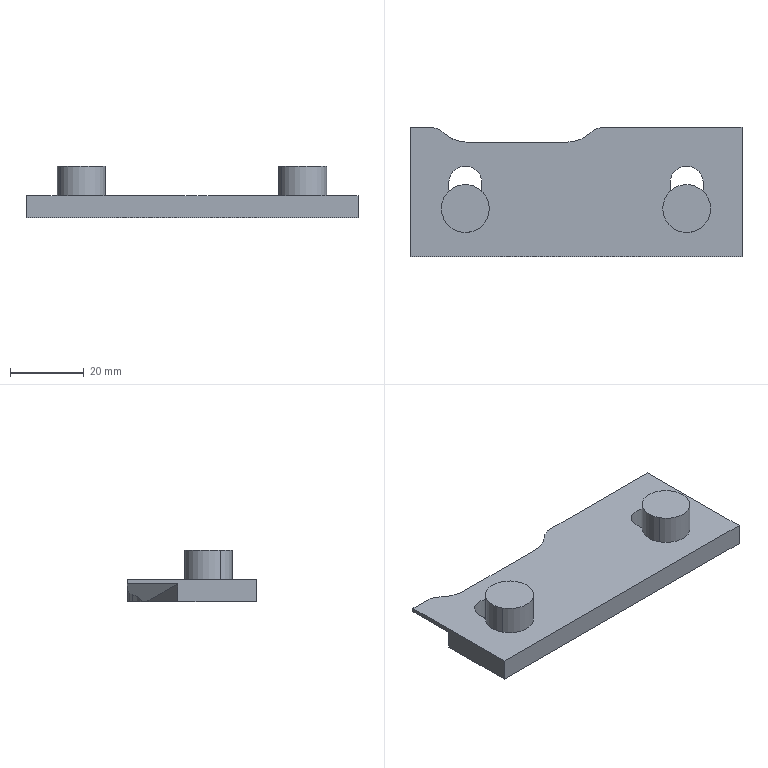Part | CATIA | 3 solids | 32 faces | box 90 x 35 x 14 mm | volume 17820 mm3 | plane 20 | cylinder 12 | commonest cylinder face diameters 9 x4 13 x4 10 x2 19 x2
STEP:
#1=CARTESIAN_POINT('',(-45.,-30.,38.));
#2=VERTEX_POINT('',#1);
#3=CARTESIAN_POINT('',(-45.,-30.,44.));
#4=VERTEX_POINT('',#3);
#5=CARTESIAN_POINT('',(-45.,-30.,41.));
#6=DIRECTION('',(0.,0.,1.));
#7=VECTOR('',#6,1.);
#8=LINE('',#5,#7);
#9=EDGE_CURVE('',#2,#4,#8,.T.);
#10=ORIENTED_EDGE('',*,*,#9,.F.);
#11=CARTESIAN_POINT('',(45.,-30.,38.));
#12=VERTEX_POINT('',#11);
#13=CARTESIAN_POINT('',(0.,-30.,38.));
#14=DIRECTION('',(1.,0.,0.));
#15=VECTOR('',#14,1.);
#16=LINE('',#13,#15);
#17=EDGE_CURVE('',#2,#12,#16,.T.);
#18=ORIENTED_EDGE('',*,*,#17,.T.);
#19=CARTESIAN_POINT('',(45.,-30.,44.));
#20=VERTEX_POINT('',#19);
#21=CARTESIAN_POINT('',(45.,-30.,41.));
#22=DIRECTION('',(0.,0.,1.));
#23=VECTOR('',#22,1.);
#24=LINE('',#21,#23);
#25=EDGE_CURVE('',#12,#20,#24,.T.);
#26=ORIENTED_EDGE('',*,*,#25,.T.);
#27=CARTESIAN_POINT('',(0.,-30.,44.));
#28=DIRECTION('',(1.,0.,0.));
#29=VECTOR('',#28,1.);
#30=LINE('',#27,#29);
#31=EDGE_CURVE('',#4,#20,#30,.T.);
#32=ORIENTED_EDGE('',*,*,#31,.F.);
#33=EDGE_LOOP('',(#10,#18,#26,#32));
#34=FACE_OUTER_BOUND('',#33,.T.);
#35=CARTESIAN_POINT('',(-45.,-30.,38.));
#36=DIRECTION('',(0.,-1.,0.));
#37=DIRECTION('',(1.,0.,0.));
#38=AXIS2_PLACEMENT_3D('',#35,#36,#37);
#39=PLANE('',#38);
#40=ADVANCED_FACE('',(#34),#39,.T.);
#41=CARTESIAN_POINT('',(45.,-8.66,42.874));
#42=VERTEX_POINT('',#41);
#43=CARTESIAN_POINT('',(45.,-8.66,38.));
#44=VERTEX_POINT('',#43);
#45=CARTESIAN_POINT('',(45.,-8.66,40.437));
#46=DIRECTION('',(0.,0.,-1.));
#47=VECTOR('',#46,1.);
#48=LINE('',#45,#47);
#49=EDGE_CURVE('',#42,#44,#48,.T.);
#50=ORIENTED_EDGE('',*,*,#49,.F.);
#51=CARTESIAN_POINT('',(45.,5.,42.874));
#52=VERTEX_POINT('',#51);
#53=CARTESIAN_POINT('',(45.,-1.83,42.874));
#54=DIRECTION('',(0.,1.,0.));
#55=VECTOR('',#54,1.);
#56=LINE('',#53,#55);
#57=EDGE_CURVE('',#42,#52,#56,.T.);
#58=ORIENTED_EDGE('',*,*,#57,.T.);
#59=CARTESIAN_POINT('',(45.,5.,44.));
#60=VERTEX_POINT('',#59);
#61=CARTESIAN_POINT('',(45.,5.,43.437));
#62=DIRECTION('',(0.,0.,1.));
#63=VECTOR('',#62,1.);
#64=LINE('',#61,#63);
#65=EDGE_CURVE('',#52,#60,#64,.T.);
#66=ORIENTED_EDGE('',*,*,#65,.T.);
#67=CARTESIAN_POINT('',(45.,-12.5,44.));
#68=DIRECTION('',(0.,-1.,0.));
#69=VECTOR('',#68,1.);
#70=LINE('',#67,#69);
#71=EDGE_CURVE('',#20,#60,#70,.F.);
#72=ORIENTED_EDGE('',*,*,#71,.F.);
#73=ORIENTED_EDGE('',*,*,#25,.F.);
#74=CARTESIAN_POINT('',(45.,-19.33,38.));
#75=DIRECTION('',(0.,-1.,0.));
#76=VECTOR('',#75,1.);
#77=LINE('',#74,#76);
#78=EDGE_CURVE('',#12,#44,#77,.F.);
#79=ORIENTED_EDGE('',*,*,#78,.T.);
#80=EDGE_LOOP('',(#50,#58,#66,#72,#73,#79));
#81=FACE_OUTER_BOUND('',#80,.T.);
#82=CARTESIAN_POINT('',(45.,5.,38.));
#83=DIRECTION('',(-1.,0.,0.));
#84=DIRECTION('',(0.,-1.,0.));
#85=AXIS2_PLACEMENT_3D('',#82,#83,#84);
#86=PLANE('',#85);
#87=ADVANCED_FACE('',(#81),#86,.F.);
#88=CARTESIAN_POINT('',(-45.,-8.66,42.874));
#89=VERTEX_POINT('',#88);
#90=CARTESIAN_POINT('',(-45.,5.,42.874));
#91=VERTEX_POINT('',#90);
#92=CARTESIAN_POINT('',(-45.,-1.83,42.874));
#93=DIRECTION('',(0.,1.,0.));
#94=VECTOR('',#93,1.);
#95=LINE('',#92,#94);
#96=EDGE_CURVE('',#89,#91,#95,.T.);
#97=ORIENTED_EDGE('',*,*,#96,.F.);
#98=CARTESIAN_POINT('',(-45.,-8.66,38.));
#99=VERTEX_POINT('',#98);
#100=CARTESIAN_POINT('',(-45.,-8.66,40.437));
#101=DIRECTION('',(0.,0.,-1.));
#102=VECTOR('',#101,1.);
#103=LINE('',#100,#102);
#104=EDGE_CURVE('',#89,#99,#103,.T.);
#105=ORIENTED_EDGE('',*,*,#104,.T.);
#106=CARTESIAN_POINT('',(-45.,-19.33,38.));
#107=DIRECTION('',(0.,1.,0.));
#108=VECTOR('',#107,1.);
#109=LINE('',#106,#108);
#110=EDGE_CURVE('',#99,#2,#109,.F.);
#111=ORIENTED_EDGE('',*,*,#110,.T.);
#112=ORIENTED_EDGE('',*,*,#9,.T.);
#113=CARTESIAN_POINT('',(-45.,5.,44.));
#114=VERTEX_POINT('',#113);
#115=CARTESIAN_POINT('',(-45.,-12.5,44.));
#116=DIRECTION('',(0.,1.,0.));
#117=VECTOR('',#116,1.);
#118=LINE('',#115,#117);
#119=EDGE_CURVE('',#114,#4,#118,.F.);
#120=ORIENTED_EDGE('',*,*,#119,.F.);
#121=CARTESIAN_POINT('',(-45.,5.,43.437));
#122=DIRECTION('',(0.,0.,1.));
#123=VECTOR('',#122,1.);
#124=LINE('',#121,#123);
#125=EDGE_CURVE('',#91,#114,#124,.T.);
#126=ORIENTED_EDGE('',*,*,#125,.F.);
#127=EDGE_LOOP('',(#97,#105,#111,#112,#120,#126));
#128=FACE_OUTER_BOUND('',#127,.T.);
#129=CARTESIAN_POINT('',(-45.,-30.,38.));
#130=DIRECTION('',(1.,0.,0.));
#131=DIRECTION('',(0.,1.,0.));
#132=AXIS2_PLACEMENT_3D('',#129,#130,#131);
#133=PLANE('',#132);
#134=ADVANCED_FACE('',(#128),#133,.F.);
#135=CARTESIAN_POINT('',(30.,0.,38.));
#136=VERTEX_POINT('',#135);
#137=CARTESIAN_POINT('',(45.,-8.66,42.874));
#138=CARTESIAN_POINT('',(30.,0.,38.));
#139=B_SPLINE_CURVE_WITH_KNOTS('',1,(#137,#138),.UNSPECIFIED.,.F.,.U.,(2,2),(-2.999,14.994),.UNSPECIFIED.);
#140=EDGE_CURVE('',#136,#42,#139,.F.);
#141=ORIENTED_EDGE('',*,*,#140,.T.);
#142=ORIENTED_EDGE('',*,*,#49,.T.);
#143=CARTESIAN_POINT('',(42.5,-7.217,38.));
#144=DIRECTION('',(0.866,-0.5,0.));
#145=VECTOR('',#144,1.);
#146=LINE('',#143,#145);
#147=EDGE_CURVE('',#136,#44,#146,.T.);
#148=ORIENTED_EDGE('',*,*,#147,.F.);
#149=EDGE_LOOP('',(#141,#142,#148));
#150=FACE_OUTER_BOUND('',#149,.T.);
#151=CARTESIAN_POINT('',(30.,0.,38.));
#152=DIRECTION('',(0.5,0.866,0.));
#153=DIRECTION('',(0.,0.,1.));
#154=AXIS2_PLACEMENT_3D('',#151,#152,#153);
#155=PLANE('',#154);
#156=ADVANCED_FACE('',(#150),#155,.T.);
#157=CARTESIAN_POINT('',(30.,5.,38.));
#158=VERTEX_POINT('',#157);
#159=CARTESIAN_POINT('',(42.5,5.,42.061));
#160=DIRECTION('',(0.9511,0.,0.309));
#161=VECTOR('',#160,1.);
#162=LINE('',#159,#161);
#163=EDGE_CURVE('',#158,#52,#162,.T.);
#164=ORIENTED_EDGE('',*,*,#163,.T.);
#165=ORIENTED_EDGE('',*,*,#57,.F.);
#166=ORIENTED_EDGE('',*,*,#140,.F.);
#167=CARTESIAN_POINT('',(30.,5.,38.));
#168=DIRECTION('',(0.,-1.,0.));
#169=VECTOR('',#168,1.);
#170=LINE('',#167,#169);
#171=EDGE_CURVE('',#136,#158,#170,.F.);
#172=ORIENTED_EDGE('',*,*,#171,.T.);
#173=EDGE_LOOP('',(#164,#165,#166,#172));
#174=FACE_OUTER_BOUND('',#173,.T.);
#175=CARTESIAN_POINT('',(30.,10.,38.));
#176=DIRECTION('',(-0.309,0.,0.9511));
#177=DIRECTION('',(0.,-1.,0.));
#178=AXIS2_PLACEMENT_3D('',#175,#176,#177);
#179=PLANE('',#178);
#180=ADVANCED_FACE('',(#174),#179,.F.);
#181=CARTESIAN_POINT('',(-30.,0.,38.));
#182=VERTEX_POINT('',#181);
#183=CARTESIAN_POINT('',(-42.5,-7.217,38.));
#184=DIRECTION('',(-0.866,-0.5,0.));
#185=VECTOR('',#184,1.);
#186=LINE('',#183,#185);
#187=EDGE_CURVE('',#182,#99,#186,.T.);
#188=ORIENTED_EDGE('',*,*,#187,.T.);
#189=ORIENTED_EDGE('',*,*,#104,.F.);
#190=CARTESIAN_POINT('',(-45.,-8.66,42.874));
#191=CARTESIAN_POINT('',(-30.,0.,38.));
#192=B_SPLINE_CURVE_WITH_KNOTS('',1,(#190,#191),.UNSPECIFIED.,.F.,.U.,(2,2),(-2.999,14.994),.UNSPECIFIED.);
#193=EDGE_CURVE('',#182,#89,#192,.F.);
#194=ORIENTED_EDGE('',*,*,#193,.F.);
#195=EDGE_LOOP('',(#188,#189,#194));
#196=FACE_OUTER_BOUND('',#195,.T.);
#197=CARTESIAN_POINT('',(-30.,0.,38.));
#198=DIRECTION('',(0.5,-0.866,0.));
#199=DIRECTION('',(0.,0.,1.));
#200=AXIS2_PLACEMENT_3D('',#197,#198,#199);
#201=PLANE('',#200);
#202=ADVANCED_FACE('',(#196),#201,.F.);
#203=CARTESIAN_POINT('',(34.5,-10.,38.));
#204=VERTEX_POINT('',#203);
#205=CARTESIAN_POINT('',(25.5,-10.,38.));
#206=VERTEX_POINT('',#205);
#207=CARTESIAN_POINT('',(30.,-10.,38.));
#208=DIRECTION('',(0.,0.,1.));
#209=AXIS2_PLACEMENT_3D('',#207,#208,$);
#210=CIRCLE('',#209,4.5);
#211=EDGE_CURVE('',#204,#206,#210,.T.);
#212=ORIENTED_EDGE('',*,*,#211,.F.);
#213=CARTESIAN_POINT('',(34.5,-10.,44.));
#214=VERTEX_POINT('',#213);
#215=CARTESIAN_POINT('',(34.5,-10.,34.));
#216=DIRECTION('',(0.,0.,1.));
#217=VECTOR('',#216,1.);
#218=LINE('',#215,#217);
#219=EDGE_CURVE('',#214,#204,#218,.F.);
#220=ORIENTED_EDGE('',*,*,#219,.F.);
#221=CARTESIAN_POINT('',(25.5,-10.,44.));
#222=VERTEX_POINT('',#221);
#223=CARTESIAN_POINT('',(30.,-10.,44.));
#224=DIRECTION('',(0.,0.,1.));
#225=AXIS2_PLACEMENT_3D('',#223,#224,$);
#226=CIRCLE('',#225,4.5);
#227=EDGE_CURVE('',#214,#222,#226,.T.);
#228=ORIENTED_EDGE('',*,*,#227,.T.);
#229=CARTESIAN_POINT('',(25.5,-10.,34.));
#230=DIRECTION('',(0.,0.,1.));
#231=VECTOR('',#230,1.);
#232=LINE('',#229,#231);
#233=EDGE_CURVE('',#222,#206,#232,.F.);
#234=ORIENTED_EDGE('',*,*,#233,.T.);
#235=EDGE_LOOP('',(#212,#220,#228,#234));
#236=FACE_OUTER_BOUND('',#235,.T.);
#237=CARTESIAN_POINT('',(30.,-10.,34.));
#238=DIRECTION('',(0.,0.,1.));
#239=DIRECTION('',(1.,0.,0.));
#240=AXIS2_PLACEMENT_3D('',#237,#238,#239);
#241=CYLINDRICAL_SURFACE('',#240,4.5);
#242=ADVANCED_FACE('',(#236),#241,.F.);
#243=ORIENTED_EDGE('',*,*,#233,.F.);
#244=CARTESIAN_POINT('',(25.5,-17.,44.));
#245=VERTEX_POINT('',#244);
#246=CARTESIAN_POINT('',(25.5,-13.5,44.));
#247=DIRECTION('',(0.,-1.,0.));
#248=VECTOR('',#247,1.);
#249=LINE('',#246,#248);
#250=EDGE_CURVE('',#222,#245,#249,.T.);
#251=ORIENTED_EDGE('',*,*,#250,.T.);
#252=CARTESIAN_POINT('',(25.5,-17.,38.));
#253=VERTEX_POINT('',#252);
#254=CARTESIAN_POINT('',(25.5,-17.,41.));
#255=DIRECTION('',(0.,0.,-1.));
#256=VECTOR('',#255,1.);
#257=LINE('',#254,#256);
#258=EDGE_CURVE('',#245,#253,#257,.T.);
#259=ORIENTED_EDGE('',*,*,#258,.T.);
#260=CARTESIAN_POINT('',(25.5,-13.5,38.));
#261=DIRECTION('',(0.,-1.,0.));
#262=VECTOR('',#261,1.);
#263=LINE('',#260,#262);
#264=EDGE_CURVE('',#206,#253,#263,.T.);
#265=ORIENTED_EDGE('',*,*,#264,.F.);
#266=EDGE_LOOP('',(#243,#251,#259,#265));
#267=FACE_OUTER_BOUND('',#266,.T.);
#268=CARTESIAN_POINT('',(25.5,-10.,44.));
#269=DIRECTION('',(1.,0.,0.));
#270=DIRECTION('',(0.,-1.,0.));
#271=AXIS2_PLACEMENT_3D('',#268,#269,#270);
#272=PLANE('',#271);
#273=ADVANCED_FACE('',(#267),#272,.T.);
#274=CARTESIAN_POINT('',(34.5,-17.,38.));
#275=VERTEX_POINT('',#274);
#276=CARTESIAN_POINT('',(34.5,-13.5,38.));
#277=DIRECTION('',(0.,-1.,0.));
#278=VECTOR('',#277,1.);
#279=LINE('',#276,#278);
#280=EDGE_CURVE('',#204,#275,#279,.T.);
#281=ORIENTED_EDGE('',*,*,#280,.T.);
#282=CARTESIAN_POINT('',(34.5,-17.,44.));
#283=VERTEX_POINT('',#282);
#284=CARTESIAN_POINT('',(34.5,-17.,41.));
#285=DIRECTION('',(0.,0.,-1.));
#286=VECTOR('',#285,1.);
#287=LINE('',#284,#286);
#288=EDGE_CURVE('',#283,#275,#287,.T.);
#289=ORIENTED_EDGE('',*,*,#288,.F.);
#290=CARTESIAN_POINT('',(34.5,-13.5,44.));
#291=DIRECTION('',(0.,-1.,0.));
#292=VECTOR('',#291,1.);
#293=LINE('',#290,#292);
#294=EDGE_CURVE('',#283,#214,#293,.F.);
#295=ORIENTED_EDGE('',*,*,#294,.T.);
#296=ORIENTED_EDGE('',*,*,#219,.T.);
#297=EDGE_LOOP('',(#281,#289,#295,#296));
#298=FACE_OUTER_BOUND('',#297,.T.);
#299=CARTESIAN_POINT('',(34.5,-10.,44.));
#300=DIRECTION('',(1.,0.,0.));
#301=DIRECTION('',(0.,-1.,0.));
#302=AXIS2_PLACEMENT_3D('',#299,#300,#301);
#303=PLANE('',#302);
#304=ADVANCED_FACE('',(#298),#303,.F.);
#305=CARTESIAN_POINT('',(30.,-17.,38.));
#306=DIRECTION('',(0.,0.,1.));
#307=AXIS2_PLACEMENT_3D('',#305,#306,$);
#308=CIRCLE('',#307,4.5);
#309=EDGE_CURVE('',#253,#275,#308,.T.);
#310=ORIENTED_EDGE('',*,*,#309,.F.);
#311=ORIENTED_EDGE('',*,*,#258,.F.);
#312=CARTESIAN_POINT('',(30.,-17.,44.));
#313=DIRECTION('',(0.,0.,1.));
#314=AXIS2_PLACEMENT_3D('',#312,#313,$);
#315=CIRCLE('',#314,4.5);
#316=EDGE_CURVE('',#245,#283,#315,.T.);
#317=ORIENTED_EDGE('',*,*,#316,.T.);
#318=ORIENTED_EDGE('',*,*,#288,.T.);
#319=EDGE_LOOP('',(#310,#311,#317,#318));
#320=FACE_OUTER_BOUND('',#319,.T.);
#321=CARTESIAN_POINT('',(30.,-17.,34.));
#322=DIRECTION('',(0.,0.,1.));
#323=DIRECTION('',(-1.,0.,0.));
#324=AXIS2_PLACEMENT_3D('',#321,#322,#323);
#325=CYLINDRICAL_SURFACE('',#324,4.5);
#326=ADVANCED_FACE('',(#320),#325,.F.);
#327=CARTESIAN_POINT('',(-25.5,-10.,38.));
#328=VERTEX_POINT('',#327);
#329=CARTESIAN_POINT('',(-25.5,-17.,38.));
#330=VERTEX_POINT('',#329);
#331=CARTESIAN_POINT('',(-25.5,-13.5,38.));
#332=DIRECTION('',(0.,-1.,0.));
#333=VECTOR('',#332,1.);
#334=LINE('',#331,#333);
#335=EDGE_CURVE('',#328,#330,#334,.T.);
#336=ORIENTED_EDGE('',*,*,#335,.T.);
#337=CARTESIAN_POINT('',(-25.5,-17.,44.));
#338=VERTEX_POINT('',#337);
#339=CARTESIAN_POINT('',(-25.5,-17.,41.));
#340=DIRECTION('',(0.,0.,-1.));
#341=VECTOR('',#340,1.);
#342=LINE('',#339,#341);
#343=EDGE_CURVE('',#338,#330,#342,.T.);
#344=ORIENTED_EDGE('',*,*,#343,.F.);
#345=CARTESIAN_POINT('',(-25.5,-10.,44.));
#346=VERTEX_POINT('',#345);
#347=CARTESIAN_POINT('',(-25.5,-13.5,44.));
#348=DIRECTION('',(0.,-1.,0.));
#349=VECTOR('',#348,1.);
#350=LINE('',#347,#349);
#351=EDGE_CURVE('',#338,#346,#350,.F.);
#352=ORIENTED_EDGE('',*,*,#351,.T.);
#353=CARTESIAN_POINT('',(-25.5,-10.,41.));
#354=DIRECTION('',(0.,0.,-1.));
#355=VECTOR('',#354,1.);
#356=LINE('',#353,#355);
#357=EDGE_CURVE('',#346,#328,#356,.T.);
#358=ORIENTED_EDGE('',*,*,#357,.T.);
#359=EDGE_LOOP('',(#336,#344,#352,#358));
#360=FACE_OUTER_BOUND('',#359,.T.);
#361=CARTESIAN_POINT('',(-25.5,-10.,44.));
#362=DIRECTION('',(1.,0.,0.));
#363=DIRECTION('',(0.,-1.,0.));
#364=AXIS2_PLACEMENT_3D('',#361,#362,#363);
#365=PLANE('',#364);
#366=ADVANCED_FACE('',(#360),#365,.F.);
#367=CARTESIAN_POINT('',(-34.5,-10.,38.));
#368=VERTEX_POINT('',#367);
#369=CARTESIAN_POINT('',(-30.,-10.,38.));
#370=DIRECTION('',(0.,0.,1.));
#371=AXIS2_PLACEMENT_3D('',#369,#370,$);
#372=CIRCLE('',#371,4.5);
#373=EDGE_CURVE('',#328,#368,#372,.T.);
#374=ORIENTED_EDGE('',*,*,#373,.F.);
#375=ORIENTED_EDGE('',*,*,#357,.F.);
#376=CARTESIAN_POINT('',(-34.5,-10.,44.));
#377=VERTEX_POINT('',#376);
#378=CARTESIAN_POINT('',(-30.,-10.,44.));
#379=DIRECTION('',(0.,0.,1.));
#380=AXIS2_PLACEMENT_3D('',#378,#379,$);
#381=CIRCLE('',#380,4.5);
#382=EDGE_CURVE('',#346,#377,#381,.T.);
#383=ORIENTED_EDGE('',*,*,#382,.T.);
#384=CARTESIAN_POINT('',(-34.5,-10.,34.));
#385=DIRECTION('',(0.,0.,1.));
#386=VECTOR('',#385,1.);
#387=LINE('',#384,#386);
#388=EDGE_CURVE('',#377,#368,#387,.F.);
#389=ORIENTED_EDGE('',*,*,#388,.T.);
#390=EDGE_LOOP('',(#374,#375,#383,#389));
#391=FACE_OUTER_BOUND('',#390,.T.);
#392=CARTESIAN_POINT('',(-30.,-10.,34.));
#393=DIRECTION('',(0.,0.,1.));
#394=DIRECTION('',(1.,0.,0.));
#395=AXIS2_PLACEMENT_3D('',#392,#393,#394);
#396=CYLINDRICAL_SURFACE('',#395,4.5);
#397=ADVANCED_FACE('',(#391),#396,.F.);
#398=CARTESIAN_POINT('',(-34.5,-17.,38.));
#399=VERTEX_POINT('',#398);
#400=CARTESIAN_POINT('',(-30.,-17.,38.));
#401=DIRECTION('',(0.,0.,1.));
#402=AXIS2_PLACEMENT_3D('',#400,#401,$);
#403=CIRCLE('',#402,4.5);
#404=EDGE_CURVE('',#399,#330,#403,.T.);
#405=ORIENTED_EDGE('',*,*,#404,.F.);
#406=CARTESIAN_POINT('',(-34.5,-17.,44.));
#407=VERTEX_POINT('',#406);
#408=CARTESIAN_POINT('',(-34.5,-17.,34.));
#409=DIRECTION('',(0.,0.,1.));
#410=VECTOR('',#409,1.);
#411=LINE('',#408,#410);
#412=EDGE_CURVE('',#407,#399,#411,.F.);
#413=ORIENTED_EDGE('',*,*,#412,.F.);
#414=CARTESIAN_POINT('',(-30.,-17.,44.));
#415=DIRECTION('',(0.,0.,1.));
#416=AXIS2_PLACEMENT_3D('',#414,#415,$);
#417=CIRCLE('',#416,4.5);
#418=EDGE_CURVE('',#407,#338,#417,.T.);
#419=ORIENTED_EDGE('',*,*,#418,.T.);
#420=ORIENTED_EDGE('',*,*,#343,.T.);
#421=EDGE_LOOP('',(#405,#413,#419,#420));
#422=FACE_OUTER_BOUND('',#421,.T.);
#423=CARTESIAN_POINT('',(-30.,-17.,34.));
#424=DIRECTION('',(0.,0.,1.));
#425=DIRECTION('',(-1.,0.,0.));
#426=AXIS2_PLACEMENT_3D('',#423,#424,#425);
#427=CYLINDRICAL_SURFACE('',#426,4.5);
#428=ADVANCED_FACE('',(#422),#427,.F.);
#429=ORIENTED_EDGE('',*,*,#388,.F.);
#430=CARTESIAN_POINT('',(-34.5,-13.5,44.));
#431=DIRECTION('',(0.,-1.,0.));
#432=VECTOR('',#431,1.);
#433=LINE('',#430,#432);
#434=EDGE_CURVE('',#377,#407,#433,.T.);
#435=ORIENTED_EDGE('',*,*,#434,.T.);
#436=ORIENTED_EDGE('',*,*,#412,.T.);
#437=CARTESIAN_POINT('',(-34.5,-13.5,38.));
#438=DIRECTION('',(0.,-1.,0.));
#439=VECTOR('',#438,1.);
#440=LINE('',#437,#439);
#441=EDGE_CURVE('',#368,#399,#440,.T.);
#442=ORIENTED_EDGE('',*,*,#441,.F.);
#443=EDGE_LOOP('',(#429,#435,#436,#442));
#444=FACE_OUTER_BOUND('',#443,.T.);
#445=CARTESIAN_POINT('',(-34.5,-10.,44.));
#446=DIRECTION('',(1.,0.,0.));
#447=DIRECTION('',(0.,-1.,0.));
#448=AXIS2_PLACEMENT_3D('',#445,#446,#447);
#449=PLANE('',#448);
#450=ADVANCED_FACE('',(#444),#449,.T.);
#451=CARTESIAN_POINT('',(-2.5,1.,38.));
#452=VERTEX_POINT('',#451);
#453=CARTESIAN_POINT('',(-29.5,1.,38.));
#454=VERTEX_POINT('',#453);
#455=CARTESIAN_POINT('',(-16.,1.,38.));
#456=DIRECTION('',(-1.,0.,0.));
#457=VECTOR('',#456,1.);
#458=LINE('',#455,#457);
#459=EDGE_CURVE('',#452,#454,#458,.T.);
#460=ORIENTED_EDGE('',*,*,#459,.T.);
#461=CARTESIAN_POINT('',(-29.5,1.,44.));
#462=VERTEX_POINT('',#461);
#463=CARTESIAN_POINT('',(-29.5,1.,41.));
#464=DIRECTION('',(0.,0.,-1.));
#465=VECTOR('',#464,1.);
#466=LINE('',#463,#465);
#467=EDGE_CURVE('',#462,#454,#466,.T.);
#468=ORIENTED_EDGE('',*,*,#467,.F.);
#469=CARTESIAN_POINT('',(-2.5,1.,44.));
#470=VERTEX_POINT('',#469);
#471=CARTESIAN_POINT('',(-16.,1.,44.));
#472=DIRECTION('',(-1.,0.,0.));
#473=VECTOR('',#472,1.);
#474=LINE('',#471,#473);
#475=EDGE_CURVE('',#470,#462,#474,.T.);
#476=ORIENTED_EDGE('',*,*,#475,.F.);
#477=CARTESIAN_POINT('',(-2.5,1.,41.));
#478=DIRECTION('',(0.,0.,-1.));
#479=VECTOR('',#478,1.);
#480=LINE('',#477,#479);
#481=EDGE_CURVE('',#470,#452,#480,.T.);
#482=ORIENTED_EDGE('',*,*,#481,.T.);
#483=EDGE_LOOP('',(#460,#468,#476,#482));
#484=FACE_OUTER_BOUND('',#483,.T.);
#485=CARTESIAN_POINT('',(-2.5,1.,44.));
#486=DIRECTION('',(0.,-1.,0.));
#487=DIRECTION('',(-1.,0.,0.));
#488=AXIS2_PLACEMENT_3D('',#485,#486,#487);
#489=PLANE('',#488);
#490=ADVANCED_FACE('',(#484),#489,.F.);
#491=CARTESIAN_POINT('',(7.5,5.,38.));
#492=VERTEX_POINT('',#491);
#493=CARTESIAN_POINT('',(4.052,3.621,38.));
#494=VERTEX_POINT('',#493);
#495=CARTESIAN_POINT('',(7.5,0.,38.));
#496=DIRECTION('',(0.,0.,1.));
#497=AXIS2_PLACEMENT_3D('',#495,#496,$);
#498=CIRCLE('',#497,5.);
#499=EDGE_CURVE('',#492,#494,#498,.T.);
#500=ORIENTED_EDGE('',*,*,#499,.F.);
#501=CARTESIAN_POINT('',(18.75,5.,38.));
#502=DIRECTION('',(-1.,0.,0.));
#503=VECTOR('',#502,1.);
#504=LINE('',#501,#503);
#505=EDGE_CURVE('',#158,#492,#504,.T.);
#506=ORIENTED_EDGE('',*,*,#505,.F.);
#507=ORIENTED_EDGE('',*,*,#171,.F.);
#508=ORIENTED_EDGE('',*,*,#147,.T.);
#509=ORIENTED_EDGE('',*,*,#78,.F.);
#510=ORIENTED_EDGE('',*,*,#17,.F.);
#511=ORIENTED_EDGE('',*,*,#110,.F.);
#512=ORIENTED_EDGE('',*,*,#187,.F.);
#513=CARTESIAN_POINT('',(-30.,1.013,38.));
#514=VERTEX_POINT('',#513);
#515=CARTESIAN_POINT('',(-30.,0.5066,38.));
#516=DIRECTION('',(0.,1.,0.));
#517=VECTOR('',#516,1.);
#518=LINE('',#515,#517);
#519=EDGE_CURVE('',#182,#514,#518,.T.);
#520=ORIENTED_EDGE('',*,*,#519,.T.);
#521=CARTESIAN_POINT('',(-29.5,10.5,38.));
#522=DIRECTION('',(0.,0.,1.));
#523=AXIS2_PLACEMENT_3D('',#521,#522,$);
#524=CIRCLE('',#523,9.5);
#525=EDGE_CURVE('',#514,#454,#524,.T.);
#526=ORIENTED_EDGE('',*,*,#525,.T.);
#527=ORIENTED_EDGE('',*,*,#459,.F.);
#528=CARTESIAN_POINT('',(-2.5,10.5,38.));
#529=DIRECTION('',(0.,0.,1.));
#530=AXIS2_PLACEMENT_3D('',#528,#529,$);
#531=CIRCLE('',#530,9.5);
#532=EDGE_CURVE('',#452,#494,#531,.T.);
#533=ORIENTED_EDGE('',*,*,#532,.T.);
#534=EDGE_LOOP('',(#500,#506,#507,#508,#509,#510,#511,#512,#520,#526,#527,#533));
#535=FACE_OUTER_BOUND('',#534,.T.);
#536=ORIENTED_EDGE('',*,*,#335,.F.);
#537=ORIENTED_EDGE('',*,*,#373,.T.);
#538=ORIENTED_EDGE('',*,*,#441,.T.);
#539=ORIENTED_EDGE('',*,*,#404,.T.);
#540=EDGE_LOOP('',(#536,#537,#538,#539));
#541=FACE_BOUND('',#540,.T.);
#542=ORIENTED_EDGE('',*,*,#211,.T.);
#543=ORIENTED_EDGE('',*,*,#264,.T.);
#544=ORIENTED_EDGE('',*,*,#309,.T.);
#545=ORIENTED_EDGE('',*,*,#280,.F.);
#546=EDGE_LOOP('',(#542,#543,#544,#545));
#547=FACE_BOUND('',#546,.T.);
#548=CARTESIAN_POINT('',(0.,0.,38.));
#549=DIRECTION('',(0.,0.,1.));
#550=DIRECTION('',(1.,0.,0.));
#551=AXIS2_PLACEMENT_3D('',#548,#549,#550);
#552=PLANE('',#551);
#553=ADVANCED_FACE('',(#535,#541,#547),#552,.F.);
#554=CARTESIAN_POINT('',(7.5,5.,44.));
#555=VERTEX_POINT('',#554);
#556=CARTESIAN_POINT('',(26.25,5.,44.));
#557=DIRECTION('',(-1.,0.,0.));
#558=VECTOR('',#557,1.);
#559=LINE('',#556,#558);
#560=EDGE_CURVE('',#60,#555,#559,.T.);
#561=ORIENTED_EDGE('',*,*,#560,.F.);
#562=ORIENTED_EDGE('',*,*,#65,.F.);
#563=ORIENTED_EDGE('',*,*,#163,.F.);
#564=ORIENTED_EDGE('',*,*,#505,.T.);
#565=CARTESIAN_POINT('',(7.5,5.,41.));
#566=DIRECTION('',(0.,0.,-1.));
#567=VECTOR('',#566,1.);
#568=LINE('',#565,#567);
#569=EDGE_CURVE('',#555,#492,#568,.T.);
#570=ORIENTED_EDGE('',*,*,#569,.F.);
#571=EDGE_LOOP('',(#561,#562,#563,#564,#570));
#572=FACE_OUTER_BOUND('',#571,.T.);
#573=CARTESIAN_POINT('',(45.,5.,38.));
#574=DIRECTION('',(0.,1.,0.));
#575=DIRECTION('',(-1.,0.,0.));
#576=AXIS2_PLACEMENT_3D('',#573,#574,#575);
#577=PLANE('',#576);
#578=ADVANCED_FACE('',(#572),#577,.T.);
#579=CARTESIAN_POINT('',(4.052,3.621,44.));
#580=VERTEX_POINT('',#579);
#581=CARTESIAN_POINT('',(4.052,3.621,34.));
#582=DIRECTION('',(0.,0.,1.));
#583=VECTOR('',#582,1.);
#584=LINE('',#581,#583);
#585=EDGE_CURVE('',#580,#494,#584,.F.);
#586=ORIENTED_EDGE('',*,*,#585,.T.);
#587=ORIENTED_EDGE('',*,*,#532,.F.);
#588=ORIENTED_EDGE('',*,*,#481,.F.);
#589=CARTESIAN_POINT('',(-2.5,10.5,44.));
#590=DIRECTION('',(0.,0.,1.));
#591=AXIS2_PLACEMENT_3D('',#589,#590,$);
#592=CIRCLE('',#591,9.5);
#593=EDGE_CURVE('',#470,#580,#592,.T.);
#594=ORIENTED_EDGE('',*,*,#593,.T.);
#595=EDGE_LOOP('',(#586,#587,#588,#594));
#596=FACE_OUTER_BOUND('',#595,.T.);
#597=CARTESIAN_POINT('',(-2.5,10.5,34.));
#598=DIRECTION('',(0.,0.,1.));
#599=DIRECTION('',(0.,-1.,0.));
#600=AXIS2_PLACEMENT_3D('',#597,#598,#599);
#601=CYLINDRICAL_SURFACE('',#600,9.5);
#602=ADVANCED_FACE('',(#596),#601,.F.);
#603=ORIENTED_EDGE('',*,*,#499,.T.);
#604=ORIENTED_EDGE('',*,*,#585,.F.);
#605=CARTESIAN_POINT('',(7.5,0.,44.));
#606=DIRECTION('',(0.,0.,-1.));
#607=AXIS2_PLACEMENT_3D('',#605,#606,$);
#608=CIRCLE('',#607,5.);
#609=EDGE_CURVE('',#580,#555,#608,.T.);
#610=ORIENTED_EDGE('',*,*,#609,.T.);
#611=ORIENTED_EDGE('',*,*,#569,.T.);
#612=EDGE_LOOP('',(#603,#604,#610,#611));
#613=FACE_OUTER_BOUND('',#612,.T.);
#614=CARTESIAN_POINT('',(7.5,0.,41.));
#615=DIRECTION('',(0.,0.,-1.));
#616=DIRECTION('',(-0.6897,0.7241,0.));
#617=AXIS2_PLACEMENT_3D('',#614,#615,#616);
#618=CYLINDRICAL_SURFACE('',#617,5.);
#619=ADVANCED_FACE('',(#613),#618,.T.);
#620=CARTESIAN_POINT('',(-36.052,3.621,39.966));
#621=VERTEX_POINT('',#620);
#622=CARTESIAN_POINT('',(-36.052,3.621,39.966));
#623=CARTESIAN_POINT('',(-34.816,2.444,39.565));
#624=CARTESIAN_POINT('',(-33.312,1.578,39.076));
#625=CARTESIAN_POINT('',(-31.665,1.101,38.541));
#626=CARTESIAN_POINT('',(-30.,1.013,38.));
#627=B_SPLINE_CURVE_WITH_KNOTS('',4,(#622,#623,#624,#625,#626),.UNSPECIFIED.,.F.,.U.,(5,5),(2.642,12.559),.UNSPECIFIED.);
#628=EDGE_CURVE('',#621,#514,#627,.T.);
#629=ORIENTED_EDGE('',*,*,#628,.T.);
#630=ORIENTED_EDGE('',*,*,#519,.F.);
#631=ORIENTED_EDGE('',*,*,#193,.T.);
#632=ORIENTED_EDGE('',*,*,#96,.T.);
#633=CARTESIAN_POINT('',(-39.5,5.,41.087));
#634=VERTEX_POINT('',#633);
#635=CARTESIAN_POINT('',(-42.5,5.,42.061));
#636=DIRECTION('',(-0.9511,0.,0.309));
#637=VECTOR('',#636,1.);
#638=LINE('',#635,#637);
#639=EDGE_CURVE('',#634,#91,#638,.T.);
#640=ORIENTED_EDGE('',*,*,#639,.F.);
#641=CARTESIAN_POINT('',(-39.5,5.,41.087));
#642=CARTESIAN_POINT('',(-38.557,5.,40.78));
#643=CARTESIAN_POINT('',(-37.613,4.763,40.474));
#644=CARTESIAN_POINT('',(-36.751,4.287,40.193));
#645=CARTESIAN_POINT('',(-36.052,3.621,39.966));
#646=B_SPLINE_CURVE_WITH_KNOTS('',4,(#641,#642,#643,#644,#645),.UNSPECIFIED.,.F.,.U.,(5,5),(0.,5.611),.UNSPECIFIED.);
#647=EDGE_CURVE('',#621,#634,#646,.F.);
#648=ORIENTED_EDGE('',*,*,#647,.F.);
#649=EDGE_LOOP('',(#629,#630,#631,#632,#640,#648));
#650=FACE_OUTER_BOUND('',#649,.T.);
#651=CARTESIAN_POINT('',(-30.,10.,38.));
#652=DIRECTION('',(-0.309,0.,-0.9511));
#653=DIRECTION('',(0.,-1.,0.));
#654=AXIS2_PLACEMENT_3D('',#651,#652,#653);
#655=PLANE('',#654);
#656=ADVANCED_FACE('',(#650),#655,.T.);
#657=ORIENTED_EDGE('',*,*,#639,.T.);
#658=ORIENTED_EDGE('',*,*,#125,.T.);
#659=CARTESIAN_POINT('',(-39.5,5.,44.));
#660=VERTEX_POINT('',#659);
#661=CARTESIAN_POINT('',(-42.25,5.,44.));
#662=DIRECTION('',(-1.,0.,0.));
#663=VECTOR('',#662,1.);
#664=LINE('',#661,#663);
#665=EDGE_CURVE('',#660,#114,#664,.T.);
#666=ORIENTED_EDGE('',*,*,#665,.F.);
#667=CARTESIAN_POINT('',(-39.5,5.,42.543));
#668=DIRECTION('',(0.,0.,-1.));
#669=VECTOR('',#668,1.);
#670=LINE('',#667,#669);
#671=EDGE_CURVE('',#660,#634,#670,.T.);
#672=ORIENTED_EDGE('',*,*,#671,.T.);
#673=EDGE_LOOP('',(#657,#658,#666,#672));
#674=FACE_OUTER_BOUND('',#673,.T.);
#675=ADVANCED_FACE('',(#674),#577,.T.);
#676=CARTESIAN_POINT('',(-36.052,3.621,44.));
#677=VERTEX_POINT('',#676);
#678=CARTESIAN_POINT('',(-36.052,3.621,34.));
#679=DIRECTION('',(0.,0.,1.));
#680=VECTOR('',#679,1.);
#681=LINE('',#678,#680);
#682=EDGE_CURVE('',#677,#621,#681,.F.);
#683=ORIENTED_EDGE('',*,*,#682,.F.);
#684=CARTESIAN_POINT('',(-29.5,10.5,44.));
#685=DIRECTION('',(0.,0.,1.));
#686=AXIS2_PLACEMENT_3D('',#684,#685,$);
#687=CIRCLE('',#686,9.5);
#688=EDGE_CURVE('',#677,#462,#687,.T.);
#689=ORIENTED_EDGE('',*,*,#688,.T.);
#690=ORIENTED_EDGE('',*,*,#467,.T.);
#691=ORIENTED_EDGE('',*,*,#525,.F.);
#692=ORIENTED_EDGE('',*,*,#628,.F.);
#693=EDGE_LOOP('',(#683,#689,#690,#691,#692));
#694=FACE_OUTER_BOUND('',#693,.T.);
#695=CARTESIAN_POINT('',(-29.5,10.5,34.));
#696=DIRECTION('',(0.,0.,1.));
#697=DIRECTION('',(0.,1.,0.));
#698=AXIS2_PLACEMENT_3D('',#695,#696,#697);
#699=CYLINDRICAL_SURFACE('',#698,9.5);
#700=ADVANCED_FACE('',(#694),#699,.F.);
#701=ORIENTED_EDGE('',*,*,#665,.T.);
#702=ORIENTED_EDGE('',*,*,#119,.T.);
#703=ORIENTED_EDGE('',*,*,#31,.T.);
#704=ORIENTED_EDGE('',*,*,#71,.T.);
#705=ORIENTED_EDGE('',*,*,#560,.T.);
#706=ORIENTED_EDGE('',*,*,#609,.F.);
#707=ORIENTED_EDGE('',*,*,#593,.F.);
#708=ORIENTED_EDGE('',*,*,#475,.T.);
#709=ORIENTED_EDGE('',*,*,#688,.F.);
#710=CARTESIAN_POINT('',(-39.5,0.,44.));
#711=DIRECTION('',(0.,0.,1.));
#712=AXIS2_PLACEMENT_3D('',#710,#711,$);
#713=CIRCLE('',#712,5.);
#714=EDGE_CURVE('',#660,#677,#713,.F.);
#715=ORIENTED_EDGE('',*,*,#714,.F.);
#716=EDGE_LOOP('',(#701,#702,#703,#704,#705,#706,#707,#708,#709,#715));
#717=FACE_OUTER_BOUND('',#716,.T.);
#718=ORIENTED_EDGE('',*,*,#351,.F.);
#719=ORIENTED_EDGE('',*,*,#418,.F.);
#720=ORIENTED_EDGE('',*,*,#434,.F.);
#721=ORIENTED_EDGE('',*,*,#382,.F.);
#722=EDGE_LOOP('',(#718,#719,#720,#721));
#723=FACE_BOUND('',#722,.T.);
#724=ORIENTED_EDGE('',*,*,#227,.F.);
#725=ORIENTED_EDGE('',*,*,#294,.F.);
#726=ORIENTED_EDGE('',*,*,#316,.F.);
#727=ORIENTED_EDGE('',*,*,#250,.F.);
#728=EDGE_LOOP('',(#724,#725,#726,#727));
#729=FACE_BOUND('',#728,.T.);
#730=CARTESIAN_POINT('',(0.,0.,44.));
#731=DIRECTION('',(0.,0.,1.));
#732=DIRECTION('',(1.,0.,0.));
#733=AXIS2_PLACEMENT_3D('',#730,#731,#732);
#734=PLANE('',#733);
#735=ADVANCED_FACE('',(#717,#723,#729),#734,.T.);
#736=ORIENTED_EDGE('',*,*,#647,.T.);
#737=ORIENTED_EDGE('',*,*,#671,.F.);
#738=ORIENTED_EDGE('',*,*,#714,.T.);
#739=ORIENTED_EDGE('',*,*,#682,.T.);
#740=EDGE_LOOP('',(#736,#737,#738,#739));
#741=FACE_OUTER_BOUND('',#740,.T.);
#742=CARTESIAN_POINT('',(-39.5,0.,41.));
#743=DIRECTION('',(0.,0.,-1.));
#744=DIRECTION('',(0.,1.,0.));
#745=AXIS2_PLACEMENT_3D('',#742,#743,#744);
#746=CYLINDRICAL_SURFACE('',#745,5.);
#747=ADVANCED_FACE('',(#741),#746,.T.);
#748=CLOSED_SHELL('',(#40,#87,#134,#156,#180,#202,#242,#273,#304,#326,#366,#397,#428,#450,#490,#553,#578,#602,#619,#656,#675,#700,#735,#747));
#749=MANIFOLD_SOLID_BREP('',#748);
#750=CARTESIAN_POINT('',(-24.296,-13.884,52.));
#751=VERTEX_POINT('',#750);
#752=CARTESIAN_POINT('',(-35.704,-20.116,52.));
#753=VERTEX_POINT('',#752);
#754=CARTESIAN_POINT('',(-30.,-17.,52.));
#755=DIRECTION('',(0.,0.,1.));
#756=AXIS2_PLACEMENT_3D('',#754,#755,$);
#757=CIRCLE('',#756,6.5);
#758=EDGE_CURVE('',#751,#753,#757,.T.);
#759=ORIENTED_EDGE('',*,*,#758,.T.);
#760=CARTESIAN_POINT('',(-30.,-17.,52.));
#761=DIRECTION('',(0.,0.,1.));
#762=AXIS2_PLACEMENT_3D('',#760,#761,$);
#763=CIRCLE('',#762,6.5);
#764=EDGE_CURVE('',#753,#751,#763,.T.);
#765=ORIENTED_EDGE('',*,*,#764,.T.);
#766=EDGE_LOOP('',(#759,#765));
#767=FACE_OUTER_BOUND('',#766,.T.);
#768=CARTESIAN_POINT('',(-30.,-17.,52.));
#769=DIRECTION('',(0.,0.,1.));
#770=DIRECTION('',(1.,0.,0.));
#771=AXIS2_PLACEMENT_3D('',#768,#769,#770);
#772=PLANE('',#771);
#773=ADVANCED_FACE('',(#767),#772,.T.);
#774=CARTESIAN_POINT('',(-35.704,-20.116,44.));
#775=VERTEX_POINT('',#774);
#776=CARTESIAN_POINT('',(-35.704,-20.116,47.8));
#777=DIRECTION('',(0.,0.,1.));
#778=VECTOR('',#777,1.);
#779=LINE('',#776,#778);
#780=EDGE_CURVE('',#753,#775,#779,.F.);
#781=ORIENTED_EDGE('',*,*,#780,.F.);
#782=ORIENTED_EDGE('',*,*,#758,.F.);
#783=CARTESIAN_POINT('',(-24.296,-13.884,44.));
#784=VERTEX_POINT('',#783);
#785=CARTESIAN_POINT('',(-24.296,-13.884,47.8));
#786=DIRECTION('',(0.,0.,1.));
#787=VECTOR('',#786,1.);
#788=LINE('',#785,#787);
#789=EDGE_CURVE('',#751,#784,#788,.F.);
#790=ORIENTED_EDGE('',*,*,#789,.T.);
#791=CARTESIAN_POINT('',(-30.,-17.,44.));
#792=DIRECTION('',(0.,0.,1.));
#793=AXIS2_PLACEMENT_3D('',#791,#792,$);
#794=CIRCLE('',#793,6.5);
#795=EDGE_CURVE('',#784,#775,#794,.T.);
#796=ORIENTED_EDGE('',*,*,#795,.T.);
#797=EDGE_LOOP('',(#781,#782,#790,#796));
#798=FACE_OUTER_BOUND('',#797,.T.);
#799=CARTESIAN_POINT('',(-30.,-17.,44.1));
#800=DIRECTION('',(0.,0.,1.));
#801=DIRECTION('',(0.8776,0.4794,0.));
#802=AXIS2_PLACEMENT_3D('',#799,#800,#801);
#803=CYLINDRICAL_SURFACE('',#802,6.5);
#804=ADVANCED_FACE('',(#798),#803,.T.);
#805=ORIENTED_EDGE('',*,*,#789,.F.);
#806=ORIENTED_EDGE('',*,*,#764,.F.);
#807=ORIENTED_EDGE('',*,*,#780,.T.);
#808=CARTESIAN_POINT('',(-30.,-17.,44.));
#809=DIRECTION('',(0.,0.,1.));
#810=AXIS2_PLACEMENT_3D('',#808,#809,$);
#811=CIRCLE('',#810,6.5);
#812=EDGE_CURVE('',#775,#784,#811,.T.);
#813=ORIENTED_EDGE('',*,*,#812,.T.);
#814=EDGE_LOOP('',(#805,#806,#807,#813));
#815=FACE_OUTER_BOUND('',#814,.T.);
#816=ADVANCED_FACE('',(#815),#803,.T.);
#817=ORIENTED_EDGE('',*,*,#795,.F.);
#818=ORIENTED_EDGE('',*,*,#812,.F.);
#819=EDGE_LOOP('',(#817,#818));
#820=FACE_OUTER_BOUND('',#819,.T.);
#821=ADVANCED_FACE('',(#820),#734,.F.);
#822=CLOSED_SHELL('',(#773,#804,#816,#821));
#823=MANIFOLD_SOLID_BREP('',#822);
#824=CARTESIAN_POINT('',(35.704,-13.884,52.));
#825=VERTEX_POINT('',#824);
#826=CARTESIAN_POINT('',(24.296,-20.116,52.));
#827=VERTEX_POINT('',#826);
#828=CARTESIAN_POINT('',(30.,-17.,52.));
#829=DIRECTION('',(0.,0.,1.));
#830=AXIS2_PLACEMENT_3D('',#828,#829,$);
#831=CIRCLE('',#830,6.5);
#832=EDGE_CURVE('',#825,#827,#831,.T.);
#833=ORIENTED_EDGE('',*,*,#832,.T.);
#834=CARTESIAN_POINT('',(30.,-17.,52.));
#835=DIRECTION('',(0.,0.,1.));
#836=AXIS2_PLACEMENT_3D('',#834,#835,$);
#837=CIRCLE('',#836,6.5);
#838=EDGE_CURVE('',#827,#825,#837,.T.);
#839=ORIENTED_EDGE('',*,*,#838,.T.);
#840=EDGE_LOOP('',(#833,#839));
#841=FACE_OUTER_BOUND('',#840,.T.);
#842=ADVANCED_FACE('',(#841),#772,.T.);
#843=CARTESIAN_POINT('',(24.296,-20.116,44.));
#844=VERTEX_POINT('',#843);
#845=CARTESIAN_POINT('',(24.296,-20.116,47.8));
#846=DIRECTION('',(0.,0.,1.));
#847=VECTOR('',#846,1.);
#848=LINE('',#845,#847);
#849=EDGE_CURVE('',#827,#844,#848,.F.);
#850=ORIENTED_EDGE('',*,*,#849,.F.);
#851=ORIENTED_EDGE('',*,*,#832,.F.);
#852=CARTESIAN_POINT('',(35.704,-13.884,44.));
#853=VERTEX_POINT('',#852);
#854=CARTESIAN_POINT('',(35.704,-13.884,47.8));
#855=DIRECTION('',(0.,0.,1.));
#856=VECTOR('',#855,1.);
#857=LINE('',#854,#856);
#858=EDGE_CURVE('',#825,#853,#857,.F.);
#859=ORIENTED_EDGE('',*,*,#858,.T.);
#860=CARTESIAN_POINT('',(30.,-17.,44.));
#861=DIRECTION('',(0.,0.,1.));
#862=AXIS2_PLACEMENT_3D('',#860,#861,$);
#863=CIRCLE('',#862,6.5);
#864=EDGE_CURVE('',#853,#844,#863,.T.);
#865=ORIENTED_EDGE('',*,*,#864,.T.);
#866=EDGE_LOOP('',(#850,#851,#859,#865));
#867=FACE_OUTER_BOUND('',#866,.T.);
#868=CARTESIAN_POINT('',(30.,-17.,44.1));
#869=DIRECTION('',(0.,0.,1.));
#870=DIRECTION('',(0.8776,0.4794,0.));
#871=AXIS2_PLACEMENT_3D('',#868,#869,#870);
#872=CYLINDRICAL_SURFACE('',#871,6.5);
#873=ADVANCED_FACE('',(#867),#872,.T.);
#874=ORIENTED_EDGE('',*,*,#858,.F.);
#875=ORIENTED_EDGE('',*,*,#838,.F.);
#876=ORIENTED_EDGE('',*,*,#849,.T.);
#877=CARTESIAN_POINT('',(30.,-17.,44.));
#878=DIRECTION('',(0.,0.,1.));
#879=AXIS2_PLACEMENT_3D('',#877,#878,$);
#880=CIRCLE('',#879,6.5);
#881=EDGE_CURVE('',#844,#853,#880,.T.);
#882=ORIENTED_EDGE('',*,*,#881,.T.);
#883=EDGE_LOOP('',(#874,#875,#876,#882));
#884=FACE_OUTER_BOUND('',#883,.T.);
#885=ADVANCED_FACE('',(#884),#872,.T.);
#886=ORIENTED_EDGE('',*,*,#864,.F.);
#887=ORIENTED_EDGE('',*,*,#881,.F.);
#888=EDGE_LOOP('',(#886,#887));
#889=FACE_OUTER_BOUND('',#888,.T.);
#890=ADVANCED_FACE('',(#889),#734,.F.);
#891=CLOSED_SHELL('',(#842,#873,#885,#890));
#892=MANIFOLD_SOLID_BREP('',#891);
#893=(LENGTH_UNIT()NAMED_UNIT(*)SI_UNIT(.MILLI.,.METRE.));
#894=UNCERTAINTY_MEASURE_WITH_UNIT(LENGTH_MEASURE(0.005),#893,'','');
#895=(NAMED_UNIT(*)PLANE_ANGLE_UNIT()SI_UNIT($,.RADIAN.));
#896=(NAMED_UNIT(*)SI_UNIT($,.STERADIAN.)SOLID_ANGLE_UNIT());
#897=(GEOMETRIC_REPRESENTATION_CONTEXT(3)GLOBAL_UNCERTAINTY_ASSIGNED_CONTEXT((#894))GLOBAL_UNIT_ASSIGNED_CONTEXT((#893,#895,#896))REPRESENTATION_CONTEXT('',''));
#898=ADVANCED_BREP_SHAPE_REPRESENTATION('',(#749,#823,#892),#897);